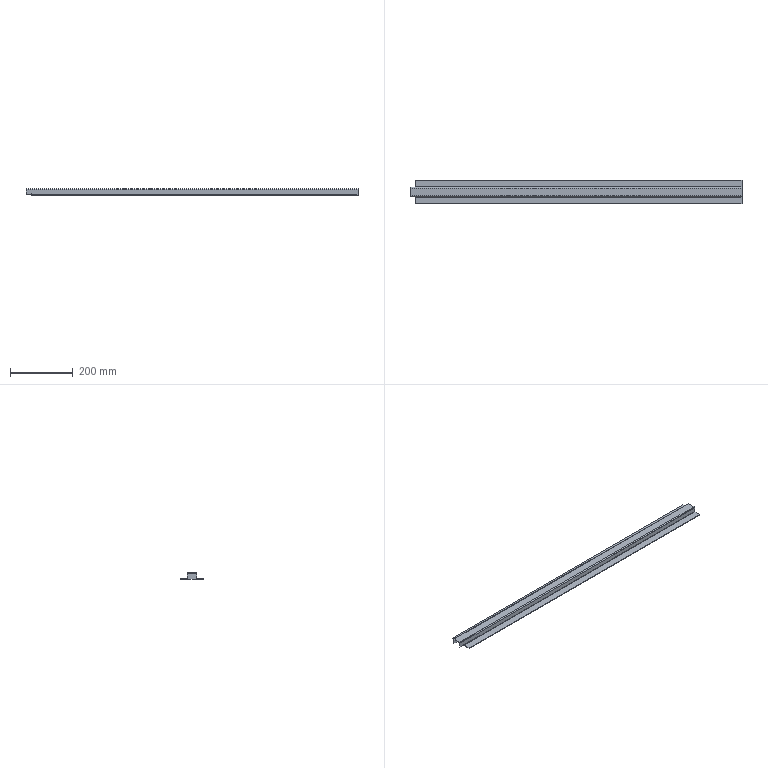Part | SolidWorks | features BaseBody 2 | 2 solids | 54 faces | box 1059 x 76 x 20 mm | volume 229133 mm3 | plane 44 | cylinder 10 | commonest cylinder face diameters 2 x6 6 x4
STEP:
#1=CARTESIAN_POINT('',(-529.5,-15.,-18.));
#2=VERTEX_POINT('',#1);
#3=CARTESIAN_POINT('',(-529.5,-13.,-18.));
#4=VERTEX_POINT('',#3);
#5=CARTESIAN_POINT('',(-529.5,-38.,-18.));
#6=DIRECTION('',(0.,1.,0.));
#7=VECTOR('',#6,1000.);
#8=LINE('',#5,#7);
#9=EDGE_CURVE('',#2,#4,#8,.T.);
#10=ORIENTED_EDGE('',*,*,#9,.T.);
#11=CARTESIAN_POINT('',(-512.5,-13.,-18.));
#12=VERTEX_POINT('',#11);
#13=CARTESIAN_POINT('',(0.,-13.,-18.));
#14=DIRECTION('',(1.,0.,0.));
#15=VECTOR('',#14,1000.);
#16=LINE('',#13,#15);
#17=EDGE_CURVE('',#4,#12,#16,.T.);
#18=ORIENTED_EDGE('',*,*,#17,.T.);
#19=CARTESIAN_POINT('',(-512.5,-15.,-18.));
#20=VERTEX_POINT('',#19);
#21=CARTESIAN_POINT('',(-512.5,-38.,-18.));
#22=DIRECTION('',(0.,1.,0.));
#23=VECTOR('',#22,1000.);
#24=LINE('',#21,#23);
#25=EDGE_CURVE('',#20,#12,#24,.T.);
#26=ORIENTED_EDGE('',*,*,#25,.F.);
#27=CARTESIAN_POINT('',(0.,-15.,-18.));
#28=DIRECTION('',(1.,0.,0.));
#29=VECTOR('',#28,1000.);
#30=LINE('',#27,#29);
#31=EDGE_CURVE('',#2,#20,#30,.T.);
#32=ORIENTED_EDGE('',*,*,#31,.F.);
#33=EDGE_LOOP('',(#10,#18,#26,#32));
#34=FACE_OUTER_BOUND('',#33,.T.);
#35=CARTESIAN_POINT('',(-529.5,-38.,-18.));
#36=DIRECTION('',(0.,0.,1.));
#37=DIRECTION('',(0.,-1.,0.));
#38=AXIS2_PLACEMENT_3D('',#35,#36,#37);
#39=PLANE('',#38);
#40=ADVANCED_FACE('',(#34),#39,.F.);
#41=CARTESIAN_POINT('',(-529.5,13.,-18.));
#42=VERTEX_POINT('',#41);
#43=CARTESIAN_POINT('',(-529.5,15.,-18.));
#44=VERTEX_POINT('',#43);
#45=CARTESIAN_POINT('',(-529.5,-38.,-18.));
#46=DIRECTION('',(0.,1.,0.));
#47=VECTOR('',#46,1000.);
#48=LINE('',#45,#47);
#49=EDGE_CURVE('',#42,#44,#48,.T.);
#50=ORIENTED_EDGE('',*,*,#49,.T.);
#51=CARTESIAN_POINT('',(-512.5,15.,-18.));
#52=VERTEX_POINT('',#51);
#53=CARTESIAN_POINT('',(-529.5,15.,-18.));
#54=DIRECTION('',(1.,0.,0.));
#55=VECTOR('',#54,1000.);
#56=LINE('',#53,#55);
#57=EDGE_CURVE('',#44,#52,#56,.T.);
#58=ORIENTED_EDGE('',*,*,#57,.T.);
#59=CARTESIAN_POINT('',(-512.5,13.,-18.));
#60=VERTEX_POINT('',#59);
#61=CARTESIAN_POINT('',(-512.5,15.,-18.));
#62=DIRECTION('',(0.,-1.,0.));
#63=VECTOR('',#62,1000.);
#64=LINE('',#61,#63);
#65=EDGE_CURVE('',#52,#60,#64,.T.);
#66=ORIENTED_EDGE('',*,*,#65,.T.);
#67=CARTESIAN_POINT('',(0.,13.,-18.));
#68=DIRECTION('',(1.,0.,0.));
#69=VECTOR('',#68,1000.);
#70=LINE('',#67,#69);
#71=EDGE_CURVE('',#42,#60,#70,.T.);
#72=ORIENTED_EDGE('',*,*,#71,.F.);
#73=EDGE_LOOP('',(#50,#58,#66,#72));
#74=FACE_OUTER_BOUND('',#73,.T.);
#75=CARTESIAN_POINT('',(-529.5,-38.,-18.));
#76=DIRECTION('',(0.,0.,1.));
#77=DIRECTION('',(0.,-1.,0.));
#78=AXIS2_PLACEMENT_3D('',#75,#76,#77);
#79=PLANE('',#78);
#80=ADVANCED_FACE('',(#74),#79,.F.);
#81=CARTESIAN_POINT('',(-511.5,38.,-18.));
#82=VERTEX_POINT('',#81);
#83=CARTESIAN_POINT('',(529.5,38.,-18.));
#84=VERTEX_POINT('',#83);
#85=CARTESIAN_POINT('',(529.5,38.,-18.));
#86=DIRECTION('',(1.,0.,0.));
#87=VECTOR('',#86,1000.);
#88=LINE('',#85,#87);
#89=EDGE_CURVE('',#82,#84,#88,.T.);
#90=ORIENTED_EDGE('',*,*,#89,.T.);
#91=CARTESIAN_POINT('',(529.5,38.,-20.));
#92=VERTEX_POINT('',#91);
#93=CARTESIAN_POINT('',(529.5,38.,-20.));
#94=DIRECTION('',(0.,0.,1.));
#95=VECTOR('',#94,1000.);
#96=LINE('',#93,#95);
#97=EDGE_CURVE('',#92,#84,#96,.T.);
#98=ORIENTED_EDGE('',*,*,#97,.F.);
#99=CARTESIAN_POINT('',(-511.5,38.,-20.));
#100=VERTEX_POINT('',#99);
#101=CARTESIAN_POINT('',(0.,38.,-20.));
#102=DIRECTION('',(1.,0.,0.));
#103=VECTOR('',#102,1000.);
#104=LINE('',#101,#103);
#105=EDGE_CURVE('',#100,#92,#104,.T.);
#106=ORIENTED_EDGE('',*,*,#105,.F.);
#107=CARTESIAN_POINT('',(-511.5,38.,-20.));
#108=DIRECTION('',(0.,0.,1.));
#109=VECTOR('',#108,1000.);
#110=LINE('',#107,#109);
#111=EDGE_CURVE('',#100,#82,#110,.T.);
#112=ORIENTED_EDGE('',*,*,#111,.T.);
#113=EDGE_LOOP('',(#90,#98,#106,#112));
#114=FACE_OUTER_BOUND('',#113,.T.);
#115=CARTESIAN_POINT('',(529.5,38.,-20.));
#116=DIRECTION('',(0.,-1.,0.));
#117=DIRECTION('',(-1.,0.,0.));
#118=AXIS2_PLACEMENT_3D('',#115,#116,#117);
#119=PLANE('',#118);
#120=ADVANCED_FACE('',(#114),#119,.F.);
#121=CARTESIAN_POINT('',(-511.5,16.,-18.));
#122=VERTEX_POINT('',#121);
#123=CARTESIAN_POINT('',(-511.5,15.,-18.));
#124=DIRECTION('',(0.,1.,0.));
#125=VECTOR('',#124,1000.);
#126=LINE('',#123,#125);
#127=EDGE_CURVE('',#122,#82,#126,.T.);
#128=ORIENTED_EDGE('',*,*,#127,.F.);
#129=CARTESIAN_POINT('',(529.5,16.,-18.));
#130=VERTEX_POINT('',#129);
#131=CARTESIAN_POINT('',(529.5,16.,-18.));
#132=DIRECTION('',(-1.,0.,0.));
#133=VECTOR('',#132,1000.);
#134=LINE('',#131,#133);
#135=EDGE_CURVE('',#130,#122,#134,.T.);
#136=ORIENTED_EDGE('',*,*,#135,.F.);
#137=CARTESIAN_POINT('',(529.5,15.,-18.));
#138=DIRECTION('',(0.,-1.,0.));
#139=VECTOR('',#138,1000.);
#140=LINE('',#137,#139);
#141=EDGE_CURVE('',#84,#130,#140,.T.);
#142=ORIENTED_EDGE('',*,*,#141,.F.);
#143=ORIENTED_EDGE('',*,*,#89,.F.);
#144=EDGE_LOOP('',(#128,#136,#142,#143));
#145=FACE_OUTER_BOUND('',#144,.T.);
#146=CARTESIAN_POINT('',(0.,0.,-18.));
#147=DIRECTION('',(0.,0.,1.));
#148=DIRECTION('',(1.,0.,0.));
#149=AXIS2_PLACEMENT_3D('',#146,#147,#148);
#150=PLANE('',#149);
#151=ADVANCED_FACE('',(#145),#150,.T.);
#152=CARTESIAN_POINT('',(-511.5,16.,-20.));
#153=VERTEX_POINT('',#152);
#154=CARTESIAN_POINT('',(529.5,16.,-20.));
#155=VERTEX_POINT('',#154);
#156=CARTESIAN_POINT('',(529.5,16.,-20.));
#157=DIRECTION('',(1.,0.,0.));
#158=VECTOR('',#157,1000.);
#159=LINE('',#156,#158);
#160=EDGE_CURVE('',#153,#155,#159,.T.);
#161=ORIENTED_EDGE('',*,*,#160,.F.);
#162=CARTESIAN_POINT('',(-511.5,0.,-20.));
#163=DIRECTION('',(0.,1.,0.));
#164=VECTOR('',#163,1000.);
#165=LINE('',#162,#164);
#166=EDGE_CURVE('',#153,#100,#165,.T.);
#167=ORIENTED_EDGE('',*,*,#166,.T.);
#168=ORIENTED_EDGE('',*,*,#105,.T.);
#169=CARTESIAN_POINT('',(529.5,0.,-20.));
#170=DIRECTION('',(0.,-1.,0.));
#171=VECTOR('',#170,1000.);
#172=LINE('',#169,#171);
#173=EDGE_CURVE('',#92,#155,#172,.T.);
#174=ORIENTED_EDGE('',*,*,#173,.T.);
#175=EDGE_LOOP('',(#161,#167,#168,#174));
#176=FACE_OUTER_BOUND('',#175,.T.);
#177=CARTESIAN_POINT('',(0.,0.,-20.));
#178=DIRECTION('',(0.,0.,1.));
#179=DIRECTION('',(1.,0.,0.));
#180=AXIS2_PLACEMENT_3D('',#177,#178,#179);
#181=PLANE('',#180);
#182=ADVANCED_FACE('',(#176),#181,.F.);
#183=CARTESIAN_POINT('',(-511.5,16.,-18.));
#184=DIRECTION('',(0.,0.,-1.));
#185=VECTOR('',#184,1000.);
#186=LINE('',#183,#185);
#187=EDGE_CURVE('',#122,#153,#186,.T.);
#188=ORIENTED_EDGE('',*,*,#187,.F.);
#189=ORIENTED_EDGE('',*,*,#127,.T.);
#190=ORIENTED_EDGE('',*,*,#111,.F.);
#191=ORIENTED_EDGE('',*,*,#166,.F.);
#192=EDGE_LOOP('',(#188,#189,#190,#191));
#193=FACE_OUTER_BOUND('',#192,.T.);
#194=CARTESIAN_POINT('',(-511.5,15.,-20.));
#195=DIRECTION('',(1.,0.,0.));
#196=DIRECTION('',(0.,1.,0.));
#197=AXIS2_PLACEMENT_3D('',#194,#195,#196);
#198=PLANE('',#197);
#199=ADVANCED_FACE('',(#193),#198,.F.);
#200=CARTESIAN_POINT('',(529.5,16.,-20.));
#201=DIRECTION('',(0.,0.,-1.));
#202=VECTOR('',#201,1000.);
#203=LINE('',#200,#202);
#204=EDGE_CURVE('',#130,#155,#203,.T.);
#205=ORIENTED_EDGE('',*,*,#204,.T.);
#206=ORIENTED_EDGE('',*,*,#173,.F.);
#207=ORIENTED_EDGE('',*,*,#97,.T.);
#208=ORIENTED_EDGE('',*,*,#141,.T.);
#209=EDGE_LOOP('',(#205,#206,#207,#208));
#210=FACE_OUTER_BOUND('',#209,.T.);
#211=CARTESIAN_POINT('',(529.5,15.,-20.));
#212=DIRECTION('',(-1.,0.,0.));
#213=DIRECTION('',(0.,0.,1.));
#214=AXIS2_PLACEMENT_3D('',#211,#212,#213);
#215=PLANE('',#214);
#216=ADVANCED_FACE('',(#210),#215,.F.);
#217=CARTESIAN_POINT('',(-511.5,15.,-17.));
#218=VERTEX_POINT('',#217);
#219=CARTESIAN_POINT('',(529.5,15.,-17.));
#220=VERTEX_POINT('',#219);
#221=CARTESIAN_POINT('',(-511.5,15.,-17.));
#222=DIRECTION('',(1.,0.,0.));
#223=VECTOR('',#222,1000.);
#224=LINE('',#221,#223);
#225=EDGE_CURVE('',#218,#220,#224,.T.);
#226=ORIENTED_EDGE('',*,*,#225,.T.);
#227=CARTESIAN_POINT('',(529.5,16.,-17.));
#228=DIRECTION('',(1.,0.,0.));
#229=DIRECTION('',(0.,0.,1.));
#230=AXIS2_PLACEMENT_3D('',#227,#228,#229);
#231=CIRCLE('',#230,1.);
#232=EDGE_CURVE('',#220,#130,#231,.T.);
#233=ORIENTED_EDGE('',*,*,#232,.T.);
#234=ORIENTED_EDGE('',*,*,#135,.T.);
#235=CARTESIAN_POINT('',(-511.5,16.,-17.));
#236=DIRECTION('',(-1.,0.,0.));
#237=DIRECTION('',(0.,0.,1.));
#238=AXIS2_PLACEMENT_3D('',#235,#236,#237);
#239=CIRCLE('',#238,1.);
#240=EDGE_CURVE('',#122,#218,#239,.T.);
#241=ORIENTED_EDGE('',*,*,#240,.T.);
#242=EDGE_LOOP('',(#226,#233,#234,#241));
#243=FACE_OUTER_BOUND('',#242,.T.);
#244=CARTESIAN_POINT('',(-511.5,16.,-17.));
#245=DIRECTION('',(-1.,0.,0.));
#246=DIRECTION('',(0.,0.,-1.));
#247=AXIS2_PLACEMENT_3D('',#244,#245,#246);
#248=CYLINDRICAL_SURFACE('',#247,1.);
#249=ADVANCED_FACE('',(#243),#248,.F.);
#250=CARTESIAN_POINT('',(-511.5,13.,-17.));
#251=VERTEX_POINT('',#250);
#252=CARTESIAN_POINT('',(529.5,13.,-17.));
#253=VERTEX_POINT('',#252);
#254=CARTESIAN_POINT('',(-511.5,13.,-17.));
#255=DIRECTION('',(1.,0.,0.));
#256=VECTOR('',#255,1000.);
#257=LINE('',#254,#256);
#258=EDGE_CURVE('',#251,#253,#257,.T.);
#259=ORIENTED_EDGE('',*,*,#258,.F.);
#260=CARTESIAN_POINT('',(-511.5,16.,-17.));
#261=DIRECTION('',(-1.,0.,0.));
#262=DIRECTION('',(0.,0.,1.));
#263=AXIS2_PLACEMENT_3D('',#260,#261,#262);
#264=CIRCLE('',#263,3.);
#265=EDGE_CURVE('',#153,#251,#264,.T.);
#266=ORIENTED_EDGE('',*,*,#265,.F.);
#267=ORIENTED_EDGE('',*,*,#160,.T.);
#268=CARTESIAN_POINT('',(529.5,16.,-17.));
#269=DIRECTION('',(1.,0.,0.));
#270=DIRECTION('',(0.,0.,1.));
#271=AXIS2_PLACEMENT_3D('',#268,#269,#270);
#272=CIRCLE('',#271,3.);
#273=EDGE_CURVE('',#253,#155,#272,.T.);
#274=ORIENTED_EDGE('',*,*,#273,.F.);
#275=EDGE_LOOP('',(#259,#266,#267,#274));
#276=FACE_OUTER_BOUND('',#275,.T.);
#277=CARTESIAN_POINT('',(-511.5,16.,-17.));
#278=DIRECTION('',(-1.,0.,0.));
#279=DIRECTION('',(0.,0.,-1.));
#280=AXIS2_PLACEMENT_3D('',#277,#278,#279);
#281=CYLINDRICAL_SURFACE('',#280,3.);
#282=ADVANCED_FACE('',(#276),#281,.T.);
#283=ORIENTED_EDGE('',*,*,#240,.F.);
#284=ORIENTED_EDGE('',*,*,#187,.T.);
#285=ORIENTED_EDGE('',*,*,#265,.T.);
#286=CARTESIAN_POINT('',(-511.5,15.,-17.));
#287=DIRECTION('',(0.,-1.,0.));
#288=VECTOR('',#287,1000.);
#289=LINE('',#286,#288);
#290=EDGE_CURVE('',#218,#251,#289,.T.);
#291=ORIENTED_EDGE('',*,*,#290,.F.);
#292=EDGE_LOOP('',(#283,#284,#285,#291));
#293=FACE_OUTER_BOUND('',#292,.T.);
#294=CARTESIAN_POINT('',(-511.5,16.,-17.));
#295=DIRECTION('',(1.,0.,0.));
#296=DIRECTION('',(0.,1.,0.));
#297=AXIS2_PLACEMENT_3D('',#294,#295,#296);
#298=PLANE('',#297);
#299=ADVANCED_FACE('',(#293),#298,.F.);
#300=ORIENTED_EDGE('',*,*,#204,.F.);
#301=ORIENTED_EDGE('',*,*,#232,.F.);
#302=CARTESIAN_POINT('',(529.5,15.,-17.));
#303=DIRECTION('',(0.,-1.,0.));
#304=VECTOR('',#303,1000.);
#305=LINE('',#302,#304);
#306=EDGE_CURVE('',#220,#253,#305,.T.);
#307=ORIENTED_EDGE('',*,*,#306,.T.);
#308=ORIENTED_EDGE('',*,*,#273,.T.);
#309=EDGE_LOOP('',(#300,#301,#307,#308));
#310=FACE_OUTER_BOUND('',#309,.T.);
#311=CARTESIAN_POINT('',(529.5,16.,-17.));
#312=DIRECTION('',(1.,0.,0.));
#313=DIRECTION('',(0.,1.,0.));
#314=AXIS2_PLACEMENT_3D('',#311,#312,#313);
#315=PLANE('',#314);
#316=ADVANCED_FACE('',(#310),#315,.T.);
#317=ORIENTED_EDGE('',*,*,#65,.F.);
#318=CARTESIAN_POINT('',(-512.5,15.,-16.));
#319=VERTEX_POINT('',#318);
#320=CARTESIAN_POINT('',(-512.5,15.,-20.));
#321=DIRECTION('',(0.,0.,1.));
#322=VECTOR('',#321,1000.);
#323=LINE('',#320,#322);
#324=EDGE_CURVE('',#52,#319,#323,.T.);
#325=ORIENTED_EDGE('',*,*,#324,.T.);
#326=CARTESIAN_POINT('',(-512.5,13.,-16.));
#327=VERTEX_POINT('',#326);
#328=CARTESIAN_POINT('',(-512.5,15.,-16.));
#329=DIRECTION('',(0.,-1.,0.));
#330=VECTOR('',#329,1000.);
#331=LINE('',#328,#330);
#332=EDGE_CURVE('',#319,#327,#331,.T.);
#333=ORIENTED_EDGE('',*,*,#332,.T.);
#334=CARTESIAN_POINT('',(-512.5,13.,0.));
#335=DIRECTION('',(0.,0.,-1.));
#336=VECTOR('',#335,1000.);
#337=LINE('',#334,#336);
#338=EDGE_CURVE('',#327,#60,#337,.T.);
#339=ORIENTED_EDGE('',*,*,#338,.T.);
#340=EDGE_LOOP('',(#317,#325,#333,#339));
#341=FACE_OUTER_BOUND('',#340,.T.);
#342=CARTESIAN_POINT('',(-512.5,15.,-20.));
#343=DIRECTION('',(1.,0.,0.));
#344=DIRECTION('',(0.,0.,1.));
#345=AXIS2_PLACEMENT_3D('',#342,#343,#344);
#346=PLANE('',#345);
#347=ADVANCED_FACE('',(#341),#346,.T.);
#348=ORIENTED_EDGE('',*,*,#290,.T.);
#349=CARTESIAN_POINT('',(-511.5,13.,-16.));
#350=VERTEX_POINT('',#349);
#351=CARTESIAN_POINT('',(-511.5,13.,0.));
#352=DIRECTION('',(0.,0.,1.));
#353=VECTOR('',#352,1000.);
#354=LINE('',#351,#353);
#355=EDGE_CURVE('',#251,#350,#354,.T.);
#356=ORIENTED_EDGE('',*,*,#355,.T.);
#357=CARTESIAN_POINT('',(-511.5,15.,-16.));
#358=VERTEX_POINT('',#357);
#359=CARTESIAN_POINT('',(-511.5,15.,-16.));
#360=DIRECTION('',(0.,-1.,0.));
#361=VECTOR('',#360,1000.);
#362=LINE('',#359,#361);
#363=EDGE_CURVE('',#358,#350,#362,.T.);
#364=ORIENTED_EDGE('',*,*,#363,.F.);
#365=CARTESIAN_POINT('',(-511.5,15.,-16.));
#366=DIRECTION('',(0.,0.,-1.));
#367=VECTOR('',#366,1000.);
#368=LINE('',#365,#367);
#369=EDGE_CURVE('',#358,#218,#368,.T.);
#370=ORIENTED_EDGE('',*,*,#369,.T.);
#371=EDGE_LOOP('',(#348,#356,#364,#370));
#372=FACE_OUTER_BOUND('',#371,.T.);
#373=CARTESIAN_POINT('',(-511.5,15.,-16.));
#374=DIRECTION('',(-1.,0.,0.));
#375=DIRECTION('',(0.,0.,1.));
#376=AXIS2_PLACEMENT_3D('',#373,#374,#375);
#377=PLANE('',#376);
#378=ADVANCED_FACE('',(#372),#377,.T.);
#379=ORIENTED_EDGE('',*,*,#363,.T.);
#380=CARTESIAN_POINT('',(0.,13.,-16.));
#381=DIRECTION('',(-1.,0.,0.));
#382=VECTOR('',#381,1000.);
#383=LINE('',#380,#382);
#384=EDGE_CURVE('',#350,#327,#383,.T.);
#385=ORIENTED_EDGE('',*,*,#384,.T.);
#386=ORIENTED_EDGE('',*,*,#332,.F.);
#387=CARTESIAN_POINT('',(-512.5,15.,-16.));
#388=DIRECTION('',(1.,0.,0.));
#389=VECTOR('',#388,1000.);
#390=LINE('',#387,#389);
#391=EDGE_CURVE('',#319,#358,#390,.T.);
#392=ORIENTED_EDGE('',*,*,#391,.T.);
#393=EDGE_LOOP('',(#379,#385,#386,#392));
#394=FACE_OUTER_BOUND('',#393,.T.);
#395=CARTESIAN_POINT('',(-512.5,15.,-16.));
#396=DIRECTION('',(0.,0.,-1.));
#397=DIRECTION('',(-1.,0.,0.));
#398=AXIS2_PLACEMENT_3D('',#395,#396,#397);
#399=PLANE('',#398);
#400=ADVANCED_FACE('',(#394),#399,.T.);
#401=CARTESIAN_POINT('',(-511.5,-38.,-18.));
#402=VERTEX_POINT('',#401);
#403=CARTESIAN_POINT('',(529.5,-38.,-18.));
#404=VERTEX_POINT('',#403);
#405=CARTESIAN_POINT('',(0.,-38.,-18.));
#406=DIRECTION('',(1.,0.,0.));
#407=VECTOR('',#406,1000.);
#408=LINE('',#405,#407);
#409=EDGE_CURVE('',#402,#404,#408,.T.);
#410=ORIENTED_EDGE('',*,*,#409,.F.);
#411=CARTESIAN_POINT('',(-511.5,-38.,-20.));
#412=VERTEX_POINT('',#411);
#413=CARTESIAN_POINT('',(-511.5,-38.,-20.));
#414=DIRECTION('',(0.,0.,1.));
#415=VECTOR('',#414,1000.);
#416=LINE('',#413,#415);
#417=EDGE_CURVE('',#412,#402,#416,.T.);
#418=ORIENTED_EDGE('',*,*,#417,.F.);
#419=CARTESIAN_POINT('',(529.5,-38.,-20.));
#420=VERTEX_POINT('',#419);
#421=CARTESIAN_POINT('',(-511.5,-38.,-20.));
#422=DIRECTION('',(1.,0.,0.));
#423=VECTOR('',#422,1000.);
#424=LINE('',#421,#423);
#425=EDGE_CURVE('',#412,#420,#424,.T.);
#426=ORIENTED_EDGE('',*,*,#425,.T.);
#427=CARTESIAN_POINT('',(529.5,-38.,-20.));
#428=DIRECTION('',(0.,0.,1.));
#429=VECTOR('',#428,1000.);
#430=LINE('',#427,#429);
#431=EDGE_CURVE('',#420,#404,#430,.T.);
#432=ORIENTED_EDGE('',*,*,#431,.T.);
#433=EDGE_LOOP('',(#410,#418,#426,#432));
#434=FACE_OUTER_BOUND('',#433,.T.);
#435=CARTESIAN_POINT('',(-511.5,-38.,-20.));
#436=DIRECTION('',(0.,-1.,0.));
#437=DIRECTION('',(0.,0.,-1.));
#438=AXIS2_PLACEMENT_3D('',#435,#436,#437);
#439=PLANE('',#438);
#440=ADVANCED_FACE('',(#434),#439,.T.);
#441=CARTESIAN_POINT('',(-511.5,-16.,-18.));
#442=VERTEX_POINT('',#441);
#443=CARTESIAN_POINT('',(529.5,-16.,-18.));
#444=VERTEX_POINT('',#443);
#445=CARTESIAN_POINT('',(-511.5,-16.,-18.));
#446=DIRECTION('',(1.,0.,0.));
#447=VECTOR('',#446,1000.);
#448=LINE('',#445,#447);
#449=EDGE_CURVE('',#442,#444,#448,.T.);
#450=ORIENTED_EDGE('',*,*,#449,.F.);
#451=CARTESIAN_POINT('',(-511.5,0.,-18.));
#452=DIRECTION('',(0.,-1.,0.));
#453=VECTOR('',#452,1000.);
#454=LINE('',#451,#453);
#455=EDGE_CURVE('',#442,#402,#454,.T.);
#456=ORIENTED_EDGE('',*,*,#455,.T.);
#457=ORIENTED_EDGE('',*,*,#409,.T.);
#458=CARTESIAN_POINT('',(529.5,0.,-18.));
#459=DIRECTION('',(0.,1.,0.));
#460=VECTOR('',#459,1000.);
#461=LINE('',#458,#460);
#462=EDGE_CURVE('',#404,#444,#461,.T.);
#463=ORIENTED_EDGE('',*,*,#462,.T.);
#464=EDGE_LOOP('',(#450,#456,#457,#463));
#465=FACE_OUTER_BOUND('',#464,.T.);
#466=CARTESIAN_POINT('',(0.,0.,-18.));
#467=DIRECTION('',(0.,0.,-1.));
#468=DIRECTION('',(-1.,0.,0.));
#469=AXIS2_PLACEMENT_3D('',#466,#467,#468);
#470=PLANE('',#469);
#471=ADVANCED_FACE('',(#465),#470,.F.);
#472=CARTESIAN_POINT('',(-511.5,-16.,-20.));
#473=VERTEX_POINT('',#472);
#474=CARTESIAN_POINT('',(-511.5,-15.,-20.));
#475=DIRECTION('',(0.,-1.,0.));
#476=VECTOR('',#475,1000.);
#477=LINE('',#474,#476);
#478=EDGE_CURVE('',#473,#412,#477,.T.);
#479=ORIENTED_EDGE('',*,*,#478,.F.);
#480=CARTESIAN_POINT('',(529.5,-16.,-20.));
#481=VERTEX_POINT('',#480);
#482=CARTESIAN_POINT('',(0.,-16.,-20.));
#483=DIRECTION('',(1.,0.,0.));
#484=VECTOR('',#483,1000.);
#485=LINE('',#482,#484);
#486=EDGE_CURVE('',#473,#481,#485,.T.);
#487=ORIENTED_EDGE('',*,*,#486,.T.);
#488=CARTESIAN_POINT('',(529.5,-38.,-20.));
#489=DIRECTION('',(0.,1.,0.));
#490=VECTOR('',#489,1000.);
#491=LINE('',#488,#490);
#492=EDGE_CURVE('',#420,#481,#491,.T.);
#493=ORIENTED_EDGE('',*,*,#492,.F.);
#494=ORIENTED_EDGE('',*,*,#425,.F.);
#495=EDGE_LOOP('',(#479,#487,#493,#494));
#496=FACE_OUTER_BOUND('',#495,.T.);
#497=CARTESIAN_POINT('',(0.,0.,-20.));
#498=DIRECTION('',(0.,0.,-1.));
#499=DIRECTION('',(-1.,0.,0.));
#500=AXIS2_PLACEMENT_3D('',#497,#498,#499);
#501=PLANE('',#500);
#502=ADVANCED_FACE('',(#496),#501,.T.);
#503=ORIENTED_EDGE('',*,*,#455,.F.);
#504=CARTESIAN_POINT('',(-511.5,-16.,-20.));
#505=DIRECTION('',(0.,0.,-1.));
#506=VECTOR('',#505,1000.);
#507=LINE('',#504,#506);
#508=EDGE_CURVE('',#442,#473,#507,.T.);
#509=ORIENTED_EDGE('',*,*,#508,.T.);
#510=ORIENTED_EDGE('',*,*,#478,.T.);
#511=ORIENTED_EDGE('',*,*,#417,.T.);
#512=EDGE_LOOP('',(#503,#509,#510,#511));
#513=FACE_OUTER_BOUND('',#512,.T.);
#514=CARTESIAN_POINT('',(-511.5,-15.,-20.));
#515=DIRECTION('',(-1.,0.,0.));
#516=DIRECTION('',(0.,1.,0.));
#517=AXIS2_PLACEMENT_3D('',#514,#515,#516);
#518=PLANE('',#517);
#519=ADVANCED_FACE('',(#513),#518,.T.);
#520=ORIENTED_EDGE('',*,*,#492,.T.);
#521=CARTESIAN_POINT('',(529.5,-16.,-18.));
#522=DIRECTION('',(0.,0.,-1.));
#523=VECTOR('',#522,1000.);
#524=LINE('',#521,#523);
#525=EDGE_CURVE('',#444,#481,#524,.T.);
#526=ORIENTED_EDGE('',*,*,#525,.F.);
#527=ORIENTED_EDGE('',*,*,#462,.F.);
#528=ORIENTED_EDGE('',*,*,#431,.F.);
#529=EDGE_LOOP('',(#520,#526,#527,#528));
#530=FACE_OUTER_BOUND('',#529,.T.);
#531=CARTESIAN_POINT('',(529.5,-38.,-20.));
#532=DIRECTION('',(1.,0.,0.));
#533=DIRECTION('',(0.,0.,-1.));
#534=AXIS2_PLACEMENT_3D('',#531,#532,#533);
#535=PLANE('',#534);
#536=ADVANCED_FACE('',(#530),#535,.T.);
#537=CARTESIAN_POINT('',(529.5,-15.,-17.));
#538=VERTEX_POINT('',#537);
#539=CARTESIAN_POINT('',(-511.5,-15.,-17.));
#540=VERTEX_POINT('',#539);
#541=CARTESIAN_POINT('',(529.5,-15.,-17.));
#542=DIRECTION('',(-1.,0.,0.));
#543=VECTOR('',#542,1000.);
#544=LINE('',#541,#543);
#545=EDGE_CURVE('',#538,#540,#544,.T.);
#546=ORIENTED_EDGE('',*,*,#545,.T.);
#547=CARTESIAN_POINT('',(-511.5,-16.,-17.));
#548=DIRECTION('',(-1.,0.,0.));
#549=DIRECTION('',(0.,0.,-1.));
#550=AXIS2_PLACEMENT_3D('',#547,#548,#549);
#551=CIRCLE('',#550,1.);
#552=EDGE_CURVE('',#540,#442,#551,.T.);
#553=ORIENTED_EDGE('',*,*,#552,.T.);
#554=ORIENTED_EDGE('',*,*,#449,.T.);
#555=CARTESIAN_POINT('',(529.5,-16.,-17.));
#556=DIRECTION('',(1.,0.,0.));
#557=DIRECTION('',(0.,0.,-1.));
#558=AXIS2_PLACEMENT_3D('',#555,#556,#557);
#559=CIRCLE('',#558,1.);
#560=EDGE_CURVE('',#444,#538,#559,.T.);
#561=ORIENTED_EDGE('',*,*,#560,.T.);
#562=EDGE_LOOP('',(#546,#553,#554,#561));
#563=FACE_OUTER_BOUND('',#562,.T.);
#564=CARTESIAN_POINT('',(529.5,-16.,-17.));
#565=DIRECTION('',(1.,0.,0.));
#566=DIRECTION('',(0.,0.,-1.));
#567=AXIS2_PLACEMENT_3D('',#564,#565,#566);
#568=CYLINDRICAL_SURFACE('',#567,1.);
#569=ADVANCED_FACE('',(#563),#568,.F.);
#570=CARTESIAN_POINT('',(529.5,-13.,-17.));
#571=VERTEX_POINT('',#570);
#572=CARTESIAN_POINT('',(-511.5,-13.,-17.));
#573=VERTEX_POINT('',#572);
#574=CARTESIAN_POINT('',(529.5,-13.,-17.));
#575=DIRECTION('',(-1.,0.,0.));
#576=VECTOR('',#575,1000.);
#577=LINE('',#574,#576);
#578=EDGE_CURVE('',#571,#573,#577,.T.);
#579=ORIENTED_EDGE('',*,*,#578,.F.);
#580=CARTESIAN_POINT('',(529.5,-16.,-17.));
#581=DIRECTION('',(1.,0.,0.));
#582=DIRECTION('',(0.,0.,-1.));
#583=AXIS2_PLACEMENT_3D('',#580,#581,#582);
#584=CIRCLE('',#583,3.);
#585=EDGE_CURVE('',#481,#571,#584,.T.);
#586=ORIENTED_EDGE('',*,*,#585,.F.);
#587=ORIENTED_EDGE('',*,*,#486,.F.);
#588=CARTESIAN_POINT('',(-511.5,-16.,-17.));
#589=DIRECTION('',(-1.,0.,0.));
#590=DIRECTION('',(0.,0.,-1.));
#591=AXIS2_PLACEMENT_3D('',#588,#589,#590);
#592=CIRCLE('',#591,3.);
#593=EDGE_CURVE('',#573,#473,#592,.T.);
#594=ORIENTED_EDGE('',*,*,#593,.F.);
#595=EDGE_LOOP('',(#579,#586,#587,#594));
#596=FACE_OUTER_BOUND('',#595,.T.);
#597=CARTESIAN_POINT('',(529.5,-16.,-17.));
#598=DIRECTION('',(1.,0.,0.));
#599=DIRECTION('',(0.,0.,-1.));
#600=AXIS2_PLACEMENT_3D('',#597,#598,#599);
#601=CYLINDRICAL_SURFACE('',#600,3.);
#602=ADVANCED_FACE('',(#596),#601,.T.);
#603=ORIENTED_EDGE('',*,*,#560,.F.);
#604=ORIENTED_EDGE('',*,*,#525,.T.);
#605=ORIENTED_EDGE('',*,*,#585,.T.);
#606=CARTESIAN_POINT('',(529.5,-15.,-17.));
#607=DIRECTION('',(0.,1.,0.));
#608=VECTOR('',#607,1000.);
#609=LINE('',#606,#608);
#610=EDGE_CURVE('',#538,#571,#609,.T.);
#611=ORIENTED_EDGE('',*,*,#610,.F.);
#612=EDGE_LOOP('',(#603,#604,#605,#611));
#613=FACE_OUTER_BOUND('',#612,.T.);
#614=CARTESIAN_POINT('',(529.5,-16.,-17.));
#615=DIRECTION('',(-1.,0.,0.));
#616=DIRECTION('',(0.,0.,1.));
#617=AXIS2_PLACEMENT_3D('',#614,#615,#616);
#618=PLANE('',#617);
#619=ADVANCED_FACE('',(#613),#618,.F.);
#620=ORIENTED_EDGE('',*,*,#508,.F.);
#621=ORIENTED_EDGE('',*,*,#552,.F.);
#622=CARTESIAN_POINT('',(-511.5,-15.,-17.));
#623=DIRECTION('',(0.,1.,0.));
#624=VECTOR('',#623,1000.);
#625=LINE('',#622,#624);
#626=EDGE_CURVE('',#540,#573,#625,.T.);
#627=ORIENTED_EDGE('',*,*,#626,.T.);
#628=ORIENTED_EDGE('',*,*,#593,.T.);
#629=EDGE_LOOP('',(#620,#621,#627,#628));
#630=FACE_OUTER_BOUND('',#629,.T.);
#631=CARTESIAN_POINT('',(-511.5,-16.,-17.));
#632=DIRECTION('',(-1.,0.,0.));
#633=DIRECTION('',(0.,0.,1.));
#634=AXIS2_PLACEMENT_3D('',#631,#632,#633);
#635=PLANE('',#634);
#636=ADVANCED_FACE('',(#630),#635,.T.);
#637=ORIENTED_EDGE('',*,*,#25,.T.);
#638=CARTESIAN_POINT('',(-512.5,-13.,-16.));
#639=VERTEX_POINT('',#638);
#640=CARTESIAN_POINT('',(-512.5,-13.,0.));
#641=DIRECTION('',(0.,0.,-1.));
#642=VECTOR('',#641,1000.);
#643=LINE('',#640,#642);
#644=EDGE_CURVE('',#639,#12,#643,.T.);
#645=ORIENTED_EDGE('',*,*,#644,.F.);
#646=CARTESIAN_POINT('',(-512.5,-15.,-16.));
#647=VERTEX_POINT('',#646);
#648=CARTESIAN_POINT('',(-512.5,-15.,-16.));
#649=DIRECTION('',(0.,1.,0.));
#650=VECTOR('',#649,1000.);
#651=LINE('',#648,#650);
#652=EDGE_CURVE('',#647,#639,#651,.T.);
#653=ORIENTED_EDGE('',*,*,#652,.F.);
#654=CARTESIAN_POINT('',(-512.5,-15.,-16.));
#655=DIRECTION('',(0.,0.,-1.));
#656=VECTOR('',#655,1000.);
#657=LINE('',#654,#656);
#658=EDGE_CURVE('',#647,#20,#657,.T.);
#659=ORIENTED_EDGE('',*,*,#658,.T.);
#660=EDGE_LOOP('',(#637,#645,#653,#659));
#661=FACE_OUTER_BOUND('',#660,.T.);
#662=CARTESIAN_POINT('',(-512.5,-15.,-16.));
#663=DIRECTION('',(1.,0.,0.));
#664=DIRECTION('',(0.,0.,1.));
#665=AXIS2_PLACEMENT_3D('',#662,#663,#664);
#666=PLANE('',#665);
#667=ADVANCED_FACE('',(#661),#666,.T.);
#668=CARTESIAN_POINT('',(-511.5,-13.,-16.));
#669=VERTEX_POINT('',#668);
#670=CARTESIAN_POINT('',(0.,-13.,-16.));
#671=DIRECTION('',(-1.,0.,0.));
#672=VECTOR('',#671,1000.);
#673=LINE('',#670,#672);
#674=EDGE_CURVE('',#669,#639,#673,.T.);
#675=ORIENTED_EDGE('',*,*,#674,.F.);
#676=CARTESIAN_POINT('',(-511.5,-15.,-16.));
#677=VERTEX_POINT('',#676);
#678=CARTESIAN_POINT('',(-511.5,-15.,-16.));
#679=DIRECTION('',(0.,1.,0.));
#680=VECTOR('',#679,1000.);
#681=LINE('',#678,#680);
#682=EDGE_CURVE('',#677,#669,#681,.T.);
#683=ORIENTED_EDGE('',*,*,#682,.F.);
#684=CARTESIAN_POINT('',(-511.5,-15.,-16.));
#685=DIRECTION('',(-1.,0.,0.));
#686=VECTOR('',#685,1000.);
#687=LINE('',#684,#686);
#688=EDGE_CURVE('',#677,#647,#687,.T.);
#689=ORIENTED_EDGE('',*,*,#688,.T.);
#690=ORIENTED_EDGE('',*,*,#652,.T.);
#691=EDGE_LOOP('',(#675,#683,#689,#690));
#692=FACE_OUTER_BOUND('',#691,.T.);
#693=CARTESIAN_POINT('',(-511.5,-15.,-16.));
#694=DIRECTION('',(0.,0.,-1.));
#695=DIRECTION('',(0.,-1.,0.));
#696=AXIS2_PLACEMENT_3D('',#693,#694,#695);
#697=PLANE('',#696);
#698=ADVANCED_FACE('',(#692),#697,.T.);
#699=CARTESIAN_POINT('',(-511.5,-13.,0.));
#700=DIRECTION('',(0.,0.,1.));
#701=VECTOR('',#700,1000.);
#702=LINE('',#699,#701);
#703=EDGE_CURVE('',#573,#669,#702,.T.);
#704=ORIENTED_EDGE('',*,*,#703,.F.);
#705=ORIENTED_EDGE('',*,*,#626,.F.);
#706=CARTESIAN_POINT('',(-511.5,-15.,-17.));
#707=DIRECTION('',(0.,0.,1.));
#708=VECTOR('',#707,1000.);
#709=LINE('',#706,#708);
#710=EDGE_CURVE('',#540,#677,#709,.T.);
#711=ORIENTED_EDGE('',*,*,#710,.T.);
#712=ORIENTED_EDGE('',*,*,#682,.T.);
#713=EDGE_LOOP('',(#704,#705,#711,#712));
#714=FACE_OUTER_BOUND('',#713,.T.);
#715=CARTESIAN_POINT('',(-511.5,-15.,-17.));
#716=DIRECTION('',(-1.,0.,0.));
#717=DIRECTION('',(0.,1.,0.));
#718=AXIS2_PLACEMENT_3D('',#715,#716,#717);
#719=PLANE('',#718);
#720=ADVANCED_FACE('',(#714),#719,.T.);
#721=ORIENTED_EDGE('',*,*,#9,.F.);
#722=CARTESIAN_POINT('',(-529.5,-15.,-3.));
#723=VERTEX_POINT('',#722);
#724=CARTESIAN_POINT('',(-529.5,-15.,-20.));
#725=DIRECTION('',(0.,0.,1.));
#726=VECTOR('',#725,1000.);
#727=LINE('',#724,#726);
#728=EDGE_CURVE('',#2,#723,#727,.T.);
#729=ORIENTED_EDGE('',*,*,#728,.T.);
#730=CARTESIAN_POINT('',(-529.5,-13.,-3.));
#731=VERTEX_POINT('',#730);
#732=CARTESIAN_POINT('',(-529.5,-13.,-3.));
#733=DIRECTION('',(0.,-1.,0.));
#734=VECTOR('',#733,1000.);
#735=LINE('',#732,#734);
#736=EDGE_CURVE('',#731,#723,#735,.T.);
#737=ORIENTED_EDGE('',*,*,#736,.F.);
#738=CARTESIAN_POINT('',(-529.5,-13.,0.));
#739=DIRECTION('',(0.,0.,1.));
#740=VECTOR('',#739,1000.);
#741=LINE('',#738,#740);
#742=EDGE_CURVE('',#4,#731,#741,.T.);
#743=ORIENTED_EDGE('',*,*,#742,.F.);
#744=EDGE_LOOP('',(#721,#729,#737,#743));
#745=FACE_OUTER_BOUND('',#744,.T.);
#746=CARTESIAN_POINT('',(-529.5,-15.,-20.));
#747=DIRECTION('',(-1.,0.,0.));
#748=DIRECTION('',(0.,0.,1.));
#749=AXIS2_PLACEMENT_3D('',#746,#747,#748);
#750=PLANE('',#749);
#751=ADVANCED_FACE('',(#745),#750,.T.);
#752=CARTESIAN_POINT('',(-529.5,-12.,-2.));
#753=VERTEX_POINT('',#752);
#754=CARTESIAN_POINT('',(529.5,-12.,-2.));
#755=VERTEX_POINT('',#754);
#756=CARTESIAN_POINT('',(-529.5,-12.,-2.));
#757=DIRECTION('',(1.,0.,0.));
#758=VECTOR('',#757,1000.);
#759=LINE('',#756,#758);
#760=EDGE_CURVE('',#753,#755,#759,.T.);
#761=ORIENTED_EDGE('',*,*,#760,.T.);
#762=CARTESIAN_POINT('',(529.5,-13.,-3.));
#763=VERTEX_POINT('',#762);
#764=CARTESIAN_POINT('',(529.5,-12.,-3.));
#765=DIRECTION('',(1.,0.,0.));
#766=DIRECTION('',(0.,0.,1.));
#767=AXIS2_PLACEMENT_3D('',#764,#765,#766);
#768=CIRCLE('',#767,1.);
#769=EDGE_CURVE('',#755,#763,#768,.T.);
#770=ORIENTED_EDGE('',*,*,#769,.T.);
#771=CARTESIAN_POINT('',(529.5,-13.,-3.));
#772=DIRECTION('',(-1.,0.,0.));
#773=VECTOR('',#772,1000.);
#774=LINE('',#771,#773);
#775=EDGE_CURVE('',#763,#731,#774,.T.);
#776=ORIENTED_EDGE('',*,*,#775,.T.);
#777=CARTESIAN_POINT('',(-529.5,-12.,-3.));
#778=DIRECTION('',(-1.,0.,0.));
#779=DIRECTION('',(0.,0.,1.));
#780=AXIS2_PLACEMENT_3D('',#777,#778,#779);
#781=CIRCLE('',#780,1.);
#782=EDGE_CURVE('',#731,#753,#781,.T.);
#783=ORIENTED_EDGE('',*,*,#782,.T.);
#784=EDGE_LOOP('',(#761,#770,#776,#783));
#785=FACE_OUTER_BOUND('',#784,.T.);
#786=CARTESIAN_POINT('',(-529.5,-12.,-3.));
#787=DIRECTION('',(-1.,0.,0.));
#788=DIRECTION('',(0.,-1.,0.));
#789=AXIS2_PLACEMENT_3D('',#786,#787,#788);
#790=CYLINDRICAL_SURFACE('',#789,1.);
#791=ADVANCED_FACE('',(#785),#790,.F.);
#792=CARTESIAN_POINT('',(-529.5,-12.,0.));
#793=VERTEX_POINT('',#792);
#794=CARTESIAN_POINT('',(529.5,-12.,0.));
#795=VERTEX_POINT('',#794);
#796=CARTESIAN_POINT('',(-529.5,-12.,0.));
#797=DIRECTION('',(1.,0.,0.));
#798=VECTOR('',#797,1000.);
#799=LINE('',#796,#798);
#800=EDGE_CURVE('',#793,#795,#799,.T.);
#801=ORIENTED_EDGE('',*,*,#800,.F.);
#802=CARTESIAN_POINT('',(-529.5,-12.,-3.));
#803=DIRECTION('',(-1.,0.,0.));
#804=DIRECTION('',(0.,0.,1.));
#805=AXIS2_PLACEMENT_3D('',#802,#803,#804);
#806=CIRCLE('',#805,3.);
#807=EDGE_CURVE('',#723,#793,#806,.T.);
#808=ORIENTED_EDGE('',*,*,#807,.F.);
#809=CARTESIAN_POINT('',(529.5,-15.,-3.));
#810=VERTEX_POINT('',#809);
#811=CARTESIAN_POINT('',(529.5,-15.,-3.));
#812=DIRECTION('',(1.,0.,0.));
#813=VECTOR('',#812,1000.);
#814=LINE('',#811,#813);
#815=EDGE_CURVE('',#723,#810,#814,.T.);
#816=ORIENTED_EDGE('',*,*,#815,.T.);
#817=CARTESIAN_POINT('',(529.5,-12.,-3.));
#818=DIRECTION('',(1.,0.,0.));
#819=DIRECTION('',(0.,0.,1.));
#820=AXIS2_PLACEMENT_3D('',#817,#818,#819);
#821=CIRCLE('',#820,3.);
#822=EDGE_CURVE('',#795,#810,#821,.T.);
#823=ORIENTED_EDGE('',*,*,#822,.F.);
#824=EDGE_LOOP('',(#801,#808,#816,#823));
#825=FACE_OUTER_BOUND('',#824,.T.);
#826=CARTESIAN_POINT('',(-529.5,-12.,-3.));
#827=DIRECTION('',(-1.,0.,0.));
#828=DIRECTION('',(0.,-1.,0.));
#829=AXIS2_PLACEMENT_3D('',#826,#827,#828);
#830=CYLINDRICAL_SURFACE('',#829,3.);
#831=ADVANCED_FACE('',(#825),#830,.T.);
#832=ORIENTED_EDGE('',*,*,#782,.F.);
#833=ORIENTED_EDGE('',*,*,#736,.T.);
#834=ORIENTED_EDGE('',*,*,#807,.T.);
#835=CARTESIAN_POINT('',(-529.5,-12.,-2.));
#836=DIRECTION('',(0.,0.,1.));
#837=VECTOR('',#836,1000.);
#838=LINE('',#835,#837);
#839=EDGE_CURVE('',#753,#793,#838,.T.);
#840=ORIENTED_EDGE('',*,*,#839,.F.);
#841=EDGE_LOOP('',(#832,#833,#834,#840));
#842=FACE_OUTER_BOUND('',#841,.T.);
#843=CARTESIAN_POINT('',(-529.5,-12.,-3.));
#844=DIRECTION('',(1.,0.,0.));
#845=DIRECTION('',(0.,1.,0.));
#846=AXIS2_PLACEMENT_3D('',#843,#844,#845);
#847=PLANE('',#846);
#848=ADVANCED_FACE('',(#842),#847,.F.);
#849=CARTESIAN_POINT('',(529.5,-15.,-3.));
#850=DIRECTION('',(0.,-1.,0.));
#851=VECTOR('',#850,1000.);
#852=LINE('',#849,#851);
#853=EDGE_CURVE('',#763,#810,#852,.T.);
#854=ORIENTED_EDGE('',*,*,#853,.F.);
#855=ORIENTED_EDGE('',*,*,#769,.F.);
#856=CARTESIAN_POINT('',(529.5,-12.,-2.));
#857=DIRECTION('',(0.,0.,1.));
#858=VECTOR('',#857,1000.);
#859=LINE('',#856,#858);
#860=EDGE_CURVE('',#755,#795,#859,.T.);
#861=ORIENTED_EDGE('',*,*,#860,.T.);
#862=ORIENTED_EDGE('',*,*,#822,.T.);
#863=EDGE_LOOP('',(#854,#855,#861,#862));
#864=FACE_OUTER_BOUND('',#863,.T.);
#865=CARTESIAN_POINT('',(529.5,-12.,-3.));
#866=DIRECTION('',(1.,0.,0.));
#867=DIRECTION('',(0.,1.,0.));
#868=AXIS2_PLACEMENT_3D('',#865,#866,#867);
#869=PLANE('',#868);
#870=ADVANCED_FACE('',(#864),#869,.T.);
#871=ORIENTED_EDGE('',*,*,#49,.F.);
#872=CARTESIAN_POINT('',(-529.5,13.,-3.));
#873=VERTEX_POINT('',#872);
#874=CARTESIAN_POINT('',(-529.5,13.,0.));
#875=DIRECTION('',(0.,0.,-1.));
#876=VECTOR('',#875,1000.);
#877=LINE('',#874,#876);
#878=EDGE_CURVE('',#873,#42,#877,.T.);
#879=ORIENTED_EDGE('',*,*,#878,.F.);
#880=CARTESIAN_POINT('',(-529.5,15.,-3.));
#881=VERTEX_POINT('',#880);
#882=CARTESIAN_POINT('',(-529.5,15.,-3.));
#883=DIRECTION('',(0.,1.,0.));
#884=VECTOR('',#883,1000.);
#885=LINE('',#882,#884);
#886=EDGE_CURVE('',#873,#881,#885,.T.);
#887=ORIENTED_EDGE('',*,*,#886,.T.);
#888=CARTESIAN_POINT('',(-529.5,15.,-20.));
#889=DIRECTION('',(0.,0.,-1.));
#890=VECTOR('',#889,1000.);
#891=LINE('',#888,#890);
#892=EDGE_CURVE('',#881,#44,#891,.T.);
#893=ORIENTED_EDGE('',*,*,#892,.T.);
#894=EDGE_LOOP('',(#871,#879,#887,#893));
#895=FACE_OUTER_BOUND('',#894,.T.);
#896=CARTESIAN_POINT('',(-529.5,15.,-20.));
#897=DIRECTION('',(-1.,0.,0.));
#898=DIRECTION('',(0.,0.,1.));
#899=AXIS2_PLACEMENT_3D('',#896,#897,#898);
#900=PLANE('',#899);
#901=ADVANCED_FACE('',(#895),#900,.T.);
#902=ORIENTED_EDGE('',*,*,#306,.F.);
#903=CARTESIAN_POINT('',(529.5,15.,-3.));
#904=VERTEX_POINT('',#903);
#905=CARTESIAN_POINT('',(529.5,15.,-2.));
#906=DIRECTION('',(0.,0.,1.));
#907=VECTOR('',#906,1000.);
#908=LINE('',#905,#907);
#909=EDGE_CURVE('',#220,#904,#908,.T.);
#910=ORIENTED_EDGE('',*,*,#909,.T.);
#911=CARTESIAN_POINT('',(529.5,13.,-3.));
#912=VERTEX_POINT('',#911);
#913=CARTESIAN_POINT('',(529.5,13.,-3.));
#914=DIRECTION('',(0.,1.,0.));
#915=VECTOR('',#914,1000.);
#916=LINE('',#913,#915);
#917=EDGE_CURVE('',#912,#904,#916,.T.);
#918=ORIENTED_EDGE('',*,*,#917,.F.);
#919=CARTESIAN_POINT('',(529.5,13.,0.));
#920=DIRECTION('',(0.,0.,1.));
#921=VECTOR('',#920,1000.);
#922=LINE('',#919,#921);
#923=EDGE_CURVE('',#253,#912,#922,.T.);
#924=ORIENTED_EDGE('',*,*,#923,.F.);
#925=EDGE_LOOP('',(#902,#910,#918,#924));
#926=FACE_OUTER_BOUND('',#925,.T.);
#927=CARTESIAN_POINT('',(529.5,15.,-2.));
#928=DIRECTION('',(1.,0.,0.));
#929=DIRECTION('',(0.,1.,0.));
#930=AXIS2_PLACEMENT_3D('',#927,#928,#929);
#931=PLANE('',#930);
#932=ADVANCED_FACE('',(#926),#931,.T.);
#933=CARTESIAN_POINT('',(529.5,12.,-2.));
#934=VERTEX_POINT('',#933);
#935=CARTESIAN_POINT('',(-529.5,12.,-2.));
#936=VERTEX_POINT('',#935);
#937=CARTESIAN_POINT('',(529.5,12.,-2.));
#938=DIRECTION('',(-1.,0.,0.));
#939=VECTOR('',#938,1000.);
#940=LINE('',#937,#939);
#941=EDGE_CURVE('',#934,#936,#940,.T.);
#942=ORIENTED_EDGE('',*,*,#941,.T.);
#943=CARTESIAN_POINT('',(-529.5,12.,-3.));
#944=DIRECTION('',(-1.,0.,0.));
#945=DIRECTION('',(0.,0.,-1.));
#946=AXIS2_PLACEMENT_3D('',#943,#944,#945);
#947=CIRCLE('',#946,1.);
#948=EDGE_CURVE('',#936,#873,#947,.T.);
#949=ORIENTED_EDGE('',*,*,#948,.T.);
#950=CARTESIAN_POINT('',(-529.5,13.,-3.));
#951=DIRECTION('',(1.,0.,0.));
#952=VECTOR('',#951,1000.);
#953=LINE('',#950,#952);
#954=EDGE_CURVE('',#873,#912,#953,.T.);
#955=ORIENTED_EDGE('',*,*,#954,.T.);
#956=CARTESIAN_POINT('',(529.5,12.,-3.));
#957=DIRECTION('',(1.,0.,0.));
#958=DIRECTION('',(0.,0.,-1.));
#959=AXIS2_PLACEMENT_3D('',#956,#957,#958);
#960=CIRCLE('',#959,1.);
#961=EDGE_CURVE('',#912,#934,#960,.T.);
#962=ORIENTED_EDGE('',*,*,#961,.T.);
#963=EDGE_LOOP('',(#942,#949,#955,#962));
#964=FACE_OUTER_BOUND('',#963,.T.);
#965=CARTESIAN_POINT('',(529.5,12.,-3.));
#966=DIRECTION('',(1.,0.,0.));
#967=DIRECTION('',(0.,1.,0.));
#968=AXIS2_PLACEMENT_3D('',#965,#966,#967);
#969=CYLINDRICAL_SURFACE('',#968,1.);
#970=ADVANCED_FACE('',(#964),#969,.F.);
#971=CARTESIAN_POINT('',(529.5,12.,0.));
#972=VERTEX_POINT('',#971);
#973=CARTESIAN_POINT('',(-529.5,12.,0.));
#974=VERTEX_POINT('',#973);
#975=CARTESIAN_POINT('',(529.5,12.,0.));
#976=DIRECTION('',(-1.,0.,0.));
#977=VECTOR('',#976,1000.);
#978=LINE('',#975,#977);
#979=EDGE_CURVE('',#972,#974,#978,.T.);
#980=ORIENTED_EDGE('',*,*,#979,.F.);
#981=CARTESIAN_POINT('',(529.5,12.,-3.));
#982=DIRECTION('',(1.,0.,0.));
#983=DIRECTION('',(0.,0.,-1.));
#984=AXIS2_PLACEMENT_3D('',#981,#982,#983);
#985=CIRCLE('',#984,3.);
#986=EDGE_CURVE('',#904,#972,#985,.T.);
#987=ORIENTED_EDGE('',*,*,#986,.F.);
#988=CARTESIAN_POINT('',(0.,15.,-3.));
#989=DIRECTION('',(1.,0.,0.));
#990=VECTOR('',#989,1000.);
#991=LINE('',#988,#990);
#992=EDGE_CURVE('',#881,#904,#991,.T.);
#993=ORIENTED_EDGE('',*,*,#992,.F.);
#994=CARTESIAN_POINT('',(-529.5,12.,-3.));
#995=DIRECTION('',(-1.,0.,0.));
#996=DIRECTION('',(0.,0.,-1.));
#997=AXIS2_PLACEMENT_3D('',#994,#995,#996);
#998=CIRCLE('',#997,3.);
#999=EDGE_CURVE('',#974,#881,#998,.T.);
#1000=ORIENTED_EDGE('',*,*,#999,.F.);
#1001=EDGE_LOOP('',(#980,#987,#993,#1000));
#1002=FACE_OUTER_BOUND('',#1001,.T.);
#1003=CARTESIAN_POINT('',(529.5,12.,-3.));
#1004=DIRECTION('',(1.,0.,0.));
#1005=DIRECTION('',(0.,1.,0.));
#1006=AXIS2_PLACEMENT_3D('',#1003,#1004,#1005);
#1007=CYLINDRICAL_SURFACE('',#1006,3.);
#1008=ADVANCED_FACE('',(#1002),#1007,.T.);
#1009=ORIENTED_EDGE('',*,*,#961,.F.);
#1010=ORIENTED_EDGE('',*,*,#917,.T.);
#1011=ORIENTED_EDGE('',*,*,#986,.T.);
#1012=CARTESIAN_POINT('',(529.5,12.,-2.));
#1013=DIRECTION('',(0.,0.,1.));
#1014=VECTOR('',#1013,1000.);
#1015=LINE('',#1012,#1014);
#1016=EDGE_CURVE('',#934,#972,#1015,.T.);
#1017=ORIENTED_EDGE('',*,*,#1016,.F.);
#1018=EDGE_LOOP('',(#1009,#1010,#1011,#1017));
#1019=FACE_OUTER_BOUND('',#1018,.T.);
#1020=CARTESIAN_POINT('',(529.5,12.,-3.));
#1021=DIRECTION('',(-1.,0.,0.));
#1022=DIRECTION('',(0.,0.,1.));
#1023=AXIS2_PLACEMENT_3D('',#1020,#1021,#1022);
#1024=PLANE('',#1023);
#1025=ADVANCED_FACE('',(#1019),#1024,.F.);
#1026=ORIENTED_EDGE('',*,*,#886,.F.);
#1027=ORIENTED_EDGE('',*,*,#948,.F.);
#1028=CARTESIAN_POINT('',(-529.5,12.,-2.));
#1029=DIRECTION('',(0.,0.,1.));
#1030=VECTOR('',#1029,1000.);
#1031=LINE('',#1028,#1030);
#1032=EDGE_CURVE('',#936,#974,#1031,.T.);
#1033=ORIENTED_EDGE('',*,*,#1032,.T.);
#1034=ORIENTED_EDGE('',*,*,#999,.T.);
#1035=EDGE_LOOP('',(#1026,#1027,#1033,#1034));
#1036=FACE_OUTER_BOUND('',#1035,.T.);
#1037=CARTESIAN_POINT('',(-529.5,12.,-3.));
#1038=DIRECTION('',(-1.,0.,0.));
#1039=DIRECTION('',(0.,0.,1.));
#1040=AXIS2_PLACEMENT_3D('',#1037,#1038,#1039);
#1041=PLANE('',#1040);
#1042=ADVANCED_FACE('',(#1036),#1041,.T.);
#1043=ORIENTED_EDGE('',*,*,#860,.F.);
#1044=CARTESIAN_POINT('',(529.5,15.,-2.));
#1045=DIRECTION('',(0.,1.,0.));
#1046=VECTOR('',#1045,1000.);
#1047=LINE('',#1044,#1046);
#1048=EDGE_CURVE('',#755,#934,#1047,.T.);
#1049=ORIENTED_EDGE('',*,*,#1048,.T.);
#1050=ORIENTED_EDGE('',*,*,#1016,.T.);
#1051=CARTESIAN_POINT('',(529.5,15.,0.));
#1052=DIRECTION('',(0.,1.,0.));
#1053=VECTOR('',#1052,1000.);
#1054=LINE('',#1051,#1053);
#1055=EDGE_CURVE('',#795,#972,#1054,.T.);
#1056=ORIENTED_EDGE('',*,*,#1055,.F.);
#1057=EDGE_LOOP('',(#1043,#1049,#1050,#1056));
#1058=FACE_OUTER_BOUND('',#1057,.T.);
#1059=CARTESIAN_POINT('',(529.5,15.,-2.));
#1060=DIRECTION('',(1.,0.,0.));
#1061=DIRECTION('',(0.,1.,0.));
#1062=AXIS2_PLACEMENT_3D('',#1059,#1060,#1061);
#1063=PLANE('',#1062);
#1064=ADVANCED_FACE('',(#1058),#1063,.T.);
#1065=CARTESIAN_POINT('',(-529.5,15.,-2.));
#1066=DIRECTION('',(0.,-1.,0.));
#1067=VECTOR('',#1066,1000.);
#1068=LINE('',#1065,#1067);
#1069=EDGE_CURVE('',#936,#753,#1068,.T.);
#1070=ORIENTED_EDGE('',*,*,#1069,.T.);
#1071=ORIENTED_EDGE('',*,*,#839,.T.);
#1072=CARTESIAN_POINT('',(-529.5,15.,0.));
#1073=DIRECTION('',(0.,-1.,0.));
#1074=VECTOR('',#1073,1000.);
#1075=LINE('',#1072,#1074);
#1076=EDGE_CURVE('',#974,#793,#1075,.T.);
#1077=ORIENTED_EDGE('',*,*,#1076,.F.);
#1078=ORIENTED_EDGE('',*,*,#1032,.F.);
#1079=EDGE_LOOP('',(#1070,#1071,#1077,#1078));
#1080=FACE_OUTER_BOUND('',#1079,.T.);
#1081=CARTESIAN_POINT('',(-529.5,15.,-2.));
#1082=DIRECTION('',(-1.,0.,0.));
#1083=DIRECTION('',(0.,0.,1.));
#1084=AXIS2_PLACEMENT_3D('',#1081,#1082,#1083);
#1085=PLANE('',#1084);
#1086=ADVANCED_FACE('',(#1080),#1085,.T.);
#1087=ORIENTED_EDGE('',*,*,#1076,.T.);
#1088=ORIENTED_EDGE('',*,*,#800,.T.);
#1089=ORIENTED_EDGE('',*,*,#1055,.T.);
#1090=ORIENTED_EDGE('',*,*,#979,.T.);
#1091=EDGE_LOOP('',(#1087,#1088,#1089,#1090));
#1092=FACE_OUTER_BOUND('',#1091,.T.);
#1093=CARTESIAN_POINT('',(0.,0.,0.));
#1094=DIRECTION('',(0.,0.,1.));
#1095=DIRECTION('',(1.,0.,0.));
#1096=AXIS2_PLACEMENT_3D('',#1093,#1094,#1095);
#1097=PLANE('',#1096);
#1098=ADVANCED_FACE('',(#1092),#1097,.T.);
#1099=ORIENTED_EDGE('',*,*,#760,.F.);
#1100=ORIENTED_EDGE('',*,*,#1069,.F.);
#1101=ORIENTED_EDGE('',*,*,#941,.F.);
#1102=ORIENTED_EDGE('',*,*,#1048,.F.);
#1103=EDGE_LOOP('',(#1099,#1100,#1101,#1102));
#1104=FACE_OUTER_BOUND('',#1103,.T.);
#1105=CARTESIAN_POINT('',(0.,0.,-2.));
#1106=DIRECTION('',(0.,0.,1.));
#1107=DIRECTION('',(1.,0.,0.));
#1108=AXIS2_PLACEMENT_3D('',#1105,#1106,#1107);
#1109=PLANE('',#1108);
#1110=ADVANCED_FACE('',(#1104),#1109,.F.);
#1111=ORIENTED_EDGE('',*,*,#17,.F.);
#1112=ORIENTED_EDGE('',*,*,#742,.T.);
#1113=ORIENTED_EDGE('',*,*,#775,.F.);
#1114=CARTESIAN_POINT('',(529.5,-13.,0.));
#1115=DIRECTION('',(0.,0.,-1.));
#1116=VECTOR('',#1115,1000.);
#1117=LINE('',#1114,#1116);
#1118=EDGE_CURVE('',#763,#571,#1117,.T.);
#1119=ORIENTED_EDGE('',*,*,#1118,.T.);
#1120=ORIENTED_EDGE('',*,*,#578,.T.);
#1121=ORIENTED_EDGE('',*,*,#703,.T.);
#1122=ORIENTED_EDGE('',*,*,#674,.T.);
#1123=ORIENTED_EDGE('',*,*,#644,.T.);
#1124=EDGE_LOOP('',(#1111,#1112,#1113,#1119,#1120,#1121,#1122,#1123));
#1125=FACE_OUTER_BOUND('',#1124,.T.);
#1126=CARTESIAN_POINT('',(0.,-13.,0.));
#1127=DIRECTION('',(0.,1.,0.));
#1128=DIRECTION('',(0.,0.,-1.));
#1129=AXIS2_PLACEMENT_3D('',#1126,#1127,#1128);
#1130=PLANE('',#1129);
#1131=ADVANCED_FACE('',(#1125),#1130,.T.);
#1132=ORIENTED_EDGE('',*,*,#728,.F.);
#1133=ORIENTED_EDGE('',*,*,#31,.T.);
#1134=ORIENTED_EDGE('',*,*,#658,.F.);
#1135=ORIENTED_EDGE('',*,*,#688,.F.);
#1136=ORIENTED_EDGE('',*,*,#710,.F.);
#1137=ORIENTED_EDGE('',*,*,#545,.F.);
#1138=CARTESIAN_POINT('',(529.5,-15.,-2.));
#1139=DIRECTION('',(0.,0.,-1.));
#1140=VECTOR('',#1139,1000.);
#1141=LINE('',#1138,#1140);
#1142=EDGE_CURVE('',#810,#538,#1141,.T.);
#1143=ORIENTED_EDGE('',*,*,#1142,.F.);
#1144=ORIENTED_EDGE('',*,*,#815,.F.);
#1145=EDGE_LOOP('',(#1132,#1133,#1134,#1135,#1136,#1137,#1143,#1144));
#1146=FACE_OUTER_BOUND('',#1145,.T.);
#1147=CARTESIAN_POINT('',(0.,-15.,0.));
#1148=DIRECTION('',(0.,1.,0.));
#1149=DIRECTION('',(0.,0.,-1.));
#1150=AXIS2_PLACEMENT_3D('',#1147,#1148,#1149);
#1151=PLANE('',#1150);
#1152=ADVANCED_FACE('',(#1146),#1151,.F.);
#1153=ORIENTED_EDGE('',*,*,#1142,.T.);
#1154=ORIENTED_EDGE('',*,*,#610,.T.);
#1155=ORIENTED_EDGE('',*,*,#1118,.F.);
#1156=ORIENTED_EDGE('',*,*,#853,.T.);
#1157=EDGE_LOOP('',(#1153,#1154,#1155,#1156));
#1158=FACE_OUTER_BOUND('',#1157,.T.);
#1159=CARTESIAN_POINT('',(529.5,-15.,-2.));
#1160=DIRECTION('',(1.,0.,0.));
#1161=DIRECTION('',(0.,1.,0.));
#1162=AXIS2_PLACEMENT_3D('',#1159,#1160,#1161);
#1163=PLANE('',#1162);
#1164=ADVANCED_FACE('',(#1158),#1163,.T.);
#1165=ORIENTED_EDGE('',*,*,#878,.T.);
#1166=ORIENTED_EDGE('',*,*,#71,.T.);
#1167=ORIENTED_EDGE('',*,*,#338,.F.);
#1168=ORIENTED_EDGE('',*,*,#384,.F.);
#1169=ORIENTED_EDGE('',*,*,#355,.F.);
#1170=ORIENTED_EDGE('',*,*,#258,.T.);
#1171=ORIENTED_EDGE('',*,*,#923,.T.);
#1172=ORIENTED_EDGE('',*,*,#954,.F.);
#1173=EDGE_LOOP('',(#1165,#1166,#1167,#1168,#1169,#1170,#1171,#1172));
#1174=FACE_OUTER_BOUND('',#1173,.T.);
#1175=CARTESIAN_POINT('',(0.,13.,0.));
#1176=DIRECTION('',(0.,1.,0.));
#1177=DIRECTION('',(0.,0.,-1.));
#1178=AXIS2_PLACEMENT_3D('',#1175,#1176,#1177);
#1179=PLANE('',#1178);
#1180=ADVANCED_FACE('',(#1174),#1179,.F.);
#1181=ORIENTED_EDGE('',*,*,#57,.F.);
#1182=ORIENTED_EDGE('',*,*,#892,.F.);
#1183=ORIENTED_EDGE('',*,*,#992,.T.);
#1184=ORIENTED_EDGE('',*,*,#909,.F.);
#1185=ORIENTED_EDGE('',*,*,#225,.F.);
#1186=ORIENTED_EDGE('',*,*,#369,.F.);
#1187=ORIENTED_EDGE('',*,*,#391,.F.);
#1188=ORIENTED_EDGE('',*,*,#324,.F.);
#1189=EDGE_LOOP('',(#1181,#1182,#1183,#1184,#1185,#1186,#1187,#1188));
#1190=FACE_OUTER_BOUND('',#1189,.T.);
#1191=CARTESIAN_POINT('',(0.,15.,0.));
#1192=DIRECTION('',(0.,1.,0.));
#1193=DIRECTION('',(0.,0.,-1.));
#1194=AXIS2_PLACEMENT_3D('',#1191,#1192,#1193);
#1195=PLANE('',#1194);
#1196=ADVANCED_FACE('',(#1190),#1195,.T.);
#1197=CLOSED_SHELL('',(#40,#80,#120,#151,#182,#199,#216,#249,#282,#299,#316,#347,#378,#400,#440,#471,#502,#519,#536,#569,#602,#619,#636,#667,#698,#720,#751,#791,#831,#848,#870,#901,#932,#970,#1008,#1025,#1042,#1064,#1086,#1098,#1110,#1131,#1152,#1164,#1180,#1196));
#1198=MANIFOLD_SOLID_BREP('',#1197);
#1199=CARTESIAN_POINT('',(529.5,-12.,-2.));
#1200=VERTEX_POINT('',#1199);
#1201=CARTESIAN_POINT('',(529.5,-13.,-3.));
#1202=VERTEX_POINT('',#1201);
#1203=CARTESIAN_POINT('',(529.5,-12.,-3.));
#1204=DIRECTION('',(1.,0.,0.));
#1205=DIRECTION('',(0.,0.,-1.));
#1206=AXIS2_PLACEMENT_3D('',#1203,#1204,#1205);
#1207=CIRCLE('',#1206,1.);
#1208=EDGE_CURVE('',#1200,#1202,#1207,.T.);
#1209=ORIENTED_EDGE('',*,*,#1208,.T.);
#1210=CARTESIAN_POINT('',(529.5,-13.,-20.));
#1211=VERTEX_POINT('',#1210);
#1212=CARTESIAN_POINT('',(529.5,-13.,-17.));
#1213=DIRECTION('',(0.,0.,-1.));
#1214=VECTOR('',#1213,1000.);
#1215=LINE('',#1212,#1214);
#1216=EDGE_CURVE('',#1202,#1211,#1215,.T.);
#1217=ORIENTED_EDGE('',*,*,#1216,.T.);
#1218=CARTESIAN_POINT('',(529.5,13.,-20.));
#1219=VERTEX_POINT('',#1218);
#1220=CARTESIAN_POINT('',(529.5,13.,-20.));
#1221=DIRECTION('',(0.,1.,0.));
#1222=VECTOR('',#1221,1000.);
#1223=LINE('',#1220,#1222);
#1224=EDGE_CURVE('',#1211,#1219,#1223,.T.);
#1225=ORIENTED_EDGE('',*,*,#1224,.T.);
#1226=CARTESIAN_POINT('',(529.5,13.,-3.));
#1227=VERTEX_POINT('',#1226);
#1228=CARTESIAN_POINT('',(529.5,13.,-17.));
#1229=DIRECTION('',(0.,0.,1.));
#1230=VECTOR('',#1229,1000.);
#1231=LINE('',#1228,#1230);
#1232=EDGE_CURVE('',#1219,#1227,#1231,.T.);
#1233=ORIENTED_EDGE('',*,*,#1232,.T.);
#1234=CARTESIAN_POINT('',(529.5,12.,-2.));
#1235=VERTEX_POINT('',#1234);
#1236=CARTESIAN_POINT('',(529.5,12.,-3.));
#1237=DIRECTION('',(1.,0.,0.));
#1238=DIRECTION('',(0.,0.,-1.));
#1239=AXIS2_PLACEMENT_3D('',#1236,#1237,#1238);
#1240=CIRCLE('',#1239,1.);
#1241=EDGE_CURVE('',#1227,#1235,#1240,.T.);
#1242=ORIENTED_EDGE('',*,*,#1241,.T.);
#1243=CARTESIAN_POINT('',(529.5,-12.,-2.));
#1244=DIRECTION('',(0.,-1.,0.));
#1245=VECTOR('',#1244,1000.);
#1246=LINE('',#1243,#1245);
#1247=EDGE_CURVE('',#1235,#1200,#1246,.T.);
#1248=ORIENTED_EDGE('',*,*,#1247,.T.);
#1249=EDGE_LOOP('',(#1209,#1217,#1225,#1233,#1242,#1248));
#1250=FACE_OUTER_BOUND('',#1249,.T.);
#1251=CARTESIAN_POINT('',(529.5,-12.,-3.));
#1252=DIRECTION('',(1.,0.,0.));
#1253=DIRECTION('',(0.,1.,0.));
#1254=AXIS2_PLACEMENT_3D('',#1251,#1252,#1253);
#1255=PLANE('',#1254);
#1256=ADVANCED_FACE('',(#1250),#1255,.T.);
#1257=CARTESIAN_POINT('',(527.5,-12.,-2.));
#1258=VERTEX_POINT('',#1257);
#1259=CARTESIAN_POINT('',(527.5,-13.,-3.));
#1260=VERTEX_POINT('',#1259);
#1261=CARTESIAN_POINT('',(527.5,-12.,-3.));
#1262=DIRECTION('',(1.,0.,0.));
#1263=DIRECTION('',(0.,0.,-1.));
#1264=AXIS2_PLACEMENT_3D('',#1261,#1262,#1263);
#1265=CIRCLE('',#1264,1.);
#1266=EDGE_CURVE('',#1258,#1260,#1265,.T.);
#1267=ORIENTED_EDGE('',*,*,#1266,.F.);
#1268=CARTESIAN_POINT('',(527.5,12.,-2.));
#1269=VERTEX_POINT('',#1268);
#1270=CARTESIAN_POINT('',(527.5,-12.,-2.));
#1271=DIRECTION('',(0.,-1.,0.));
#1272=VECTOR('',#1271,1000.);
#1273=LINE('',#1270,#1272);
#1274=EDGE_CURVE('',#1269,#1258,#1273,.T.);
#1275=ORIENTED_EDGE('',*,*,#1274,.F.);
#1276=CARTESIAN_POINT('',(527.5,13.,-3.));
#1277=VERTEX_POINT('',#1276);
#1278=CARTESIAN_POINT('',(527.5,12.,-3.));
#1279=DIRECTION('',(1.,0.,0.));
#1280=DIRECTION('',(0.,0.,-1.));
#1281=AXIS2_PLACEMENT_3D('',#1278,#1279,#1280);
#1282=CIRCLE('',#1281,1.);
#1283=EDGE_CURVE('',#1277,#1269,#1282,.T.);
#1284=ORIENTED_EDGE('',*,*,#1283,.F.);
#1285=CARTESIAN_POINT('',(527.5,13.,-20.));
#1286=VERTEX_POINT('',#1285);
#1287=CARTESIAN_POINT('',(527.5,13.,-17.));
#1288=DIRECTION('',(0.,0.,1.));
#1289=VECTOR('',#1288,1000.);
#1290=LINE('',#1287,#1289);
#1291=EDGE_CURVE('',#1286,#1277,#1290,.T.);
#1292=ORIENTED_EDGE('',*,*,#1291,.F.);
#1293=CARTESIAN_POINT('',(527.5,-13.,-20.));
#1294=VERTEX_POINT('',#1293);
#1295=CARTESIAN_POINT('',(527.5,13.,-20.));
#1296=DIRECTION('',(0.,1.,0.));
#1297=VECTOR('',#1296,1000.);
#1298=LINE('',#1295,#1297);
#1299=EDGE_CURVE('',#1294,#1286,#1298,.T.);
#1300=ORIENTED_EDGE('',*,*,#1299,.F.);
#1301=CARTESIAN_POINT('',(527.5,-13.,-3.));
#1302=DIRECTION('',(0.,0.,-1.));
#1303=VECTOR('',#1302,1000.);
#1304=LINE('',#1301,#1303);
#1305=EDGE_CURVE('',#1260,#1294,#1304,.T.);
#1306=ORIENTED_EDGE('',*,*,#1305,.F.);
#1307=EDGE_LOOP('',(#1267,#1275,#1284,#1292,#1300,#1306));
#1308=FACE_OUTER_BOUND('',#1307,.T.);
#1309=CARTESIAN_POINT('',(527.5,-12.,-3.));
#1310=DIRECTION('',(1.,0.,0.));
#1311=DIRECTION('',(0.,1.,0.));
#1312=AXIS2_PLACEMENT_3D('',#1309,#1310,#1311);
#1313=PLANE('',#1312);
#1314=ADVANCED_FACE('',(#1308),#1313,.F.);
#1315=ORIENTED_EDGE('',*,*,#1216,.F.);
#1316=CARTESIAN_POINT('',(527.5,-13.,-3.));
#1317=DIRECTION('',(1.,0.,0.));
#1318=VECTOR('',#1317,1000.);
#1319=LINE('',#1316,#1318);
#1320=EDGE_CURVE('',#1260,#1202,#1319,.T.);
#1321=ORIENTED_EDGE('',*,*,#1320,.F.);
#1322=ORIENTED_EDGE('',*,*,#1305,.T.);
#1323=CARTESIAN_POINT('',(527.5,-13.,-20.));
#1324=DIRECTION('',(1.,0.,0.));
#1325=VECTOR('',#1324,1000.);
#1326=LINE('',#1323,#1325);
#1327=EDGE_CURVE('',#1294,#1211,#1326,.T.);
#1328=ORIENTED_EDGE('',*,*,#1327,.T.);
#1329=EDGE_LOOP('',(#1315,#1321,#1322,#1328));
#1330=FACE_OUTER_BOUND('',#1329,.T.);
#1331=CARTESIAN_POINT('',(527.5,-13.,-17.));
#1332=DIRECTION('',(0.,-1.,0.));
#1333=DIRECTION('',(0.,0.,-1.));
#1334=AXIS2_PLACEMENT_3D('',#1331,#1332,#1333);
#1335=PLANE('',#1334);
#1336=ADVANCED_FACE('',(#1330),#1335,.T.);
#1337=ORIENTED_EDGE('',*,*,#1224,.F.);
#1338=ORIENTED_EDGE('',*,*,#1327,.F.);
#1339=ORIENTED_EDGE('',*,*,#1299,.T.);
#1340=CARTESIAN_POINT('',(527.5,13.,-20.));
#1341=DIRECTION('',(1.,0.,0.));
#1342=VECTOR('',#1341,1000.);
#1343=LINE('',#1340,#1342);
#1344=EDGE_CURVE('',#1286,#1219,#1343,.T.);
#1345=ORIENTED_EDGE('',*,*,#1344,.T.);
#1346=EDGE_LOOP('',(#1337,#1338,#1339,#1345));
#1347=FACE_OUTER_BOUND('',#1346,.T.);
#1348=CARTESIAN_POINT('',(527.5,13.,-20.));
#1349=DIRECTION('',(0.,0.,-1.));
#1350=DIRECTION('',(0.,-1.,0.));
#1351=AXIS2_PLACEMENT_3D('',#1348,#1349,#1350);
#1352=PLANE('',#1351);
#1353=ADVANCED_FACE('',(#1347),#1352,.T.);
#1354=ORIENTED_EDGE('',*,*,#1232,.F.);
#1355=ORIENTED_EDGE('',*,*,#1344,.F.);
#1356=ORIENTED_EDGE('',*,*,#1291,.T.);
#1357=CARTESIAN_POINT('',(527.5,13.,-3.));
#1358=DIRECTION('',(1.,0.,0.));
#1359=VECTOR('',#1358,1000.);
#1360=LINE('',#1357,#1359);
#1361=EDGE_CURVE('',#1277,#1227,#1360,.T.);
#1362=ORIENTED_EDGE('',*,*,#1361,.T.);
#1363=EDGE_LOOP('',(#1354,#1355,#1356,#1362));
#1364=FACE_OUTER_BOUND('',#1363,.T.);
#1365=CARTESIAN_POINT('',(527.5,13.,-17.));
#1366=DIRECTION('',(0.,1.,0.));
#1367=DIRECTION('',(0.,0.,-1.));
#1368=AXIS2_PLACEMENT_3D('',#1365,#1366,#1367);
#1369=PLANE('',#1368);
#1370=ADVANCED_FACE('',(#1364),#1369,.T.);
#1371=ORIENTED_EDGE('',*,*,#1241,.F.);
#1372=ORIENTED_EDGE('',*,*,#1361,.F.);
#1373=ORIENTED_EDGE('',*,*,#1283,.T.);
#1374=CARTESIAN_POINT('',(527.5,12.,-2.));
#1375=DIRECTION('',(1.,0.,0.));
#1376=VECTOR('',#1375,1000.);
#1377=LINE('',#1374,#1376);
#1378=EDGE_CURVE('',#1269,#1235,#1377,.T.);
#1379=ORIENTED_EDGE('',*,*,#1378,.T.);
#1380=EDGE_LOOP('',(#1371,#1372,#1373,#1379));
#1381=FACE_OUTER_BOUND('',#1380,.T.);
#1382=CARTESIAN_POINT('',(527.5,12.,-3.));
#1383=DIRECTION('',(1.,0.,0.));
#1384=DIRECTION('',(0.,0.,-1.));
#1385=AXIS2_PLACEMENT_3D('',#1382,#1383,#1384);
#1386=CYLINDRICAL_SURFACE('',#1385,1.);
#1387=ADVANCED_FACE('',(#1381),#1386,.T.);
#1388=ORIENTED_EDGE('',*,*,#1247,.F.);
#1389=ORIENTED_EDGE('',*,*,#1378,.F.);
#1390=ORIENTED_EDGE('',*,*,#1274,.T.);
#1391=CARTESIAN_POINT('',(527.5,-12.,-2.));
#1392=DIRECTION('',(1.,0.,0.));
#1393=VECTOR('',#1392,1000.);
#1394=LINE('',#1391,#1393);
#1395=EDGE_CURVE('',#1258,#1200,#1394,.T.);
#1396=ORIENTED_EDGE('',*,*,#1395,.T.);
#1397=EDGE_LOOP('',(#1388,#1389,#1390,#1396));
#1398=FACE_OUTER_BOUND('',#1397,.T.);
#1399=CARTESIAN_POINT('',(527.5,-12.,-2.));
#1400=DIRECTION('',(0.,0.,1.));
#1401=DIRECTION('',(0.,-1.,0.));
#1402=AXIS2_PLACEMENT_3D('',#1399,#1400,#1401);
#1403=PLANE('',#1402);
#1404=ADVANCED_FACE('',(#1398),#1403,.T.);
#1405=ORIENTED_EDGE('',*,*,#1208,.F.);
#1406=ORIENTED_EDGE('',*,*,#1395,.F.);
#1407=ORIENTED_EDGE('',*,*,#1266,.T.);
#1408=ORIENTED_EDGE('',*,*,#1320,.T.);
#1409=EDGE_LOOP('',(#1405,#1406,#1407,#1408));
#1410=FACE_OUTER_BOUND('',#1409,.T.);
#1411=CARTESIAN_POINT('',(527.5,-12.,-3.));
#1412=DIRECTION('',(1.,0.,0.));
#1413=DIRECTION('',(0.,0.,-1.));
#1414=AXIS2_PLACEMENT_3D('',#1411,#1412,#1413);
#1415=CYLINDRICAL_SURFACE('',#1414,1.);
#1416=ADVANCED_FACE('',(#1410),#1415,.T.);
#1417=CLOSED_SHELL('',(#1256,#1314,#1336,#1353,#1370,#1387,#1404,#1416));
#1418=MANIFOLD_SOLID_BREP('',#1417);
#1419=CARTESIAN_POINT('',(0.,0.,0.));
#1420=DIRECTION('',(0.,0.,1.));
#1421=DIRECTION('',(1.,0.,0.));
#1422=AXIS2_PLACEMENT_3D('',#1419,#1420,#1421);
#1423=(LENGTH_UNIT()NAMED_UNIT(*)SI_UNIT(.MILLI.,.METRE.));
#1424=UNCERTAINTY_MEASURE_WITH_UNIT(LENGTH_MEASURE(0.00001),#1423,'','');
#1425=(NAMED_UNIT(*)PLANE_ANGLE_UNIT()SI_UNIT($,.RADIAN.));
#1426=(NAMED_UNIT(*)SI_UNIT($,.STERADIAN.)SOLID_ANGLE_UNIT());
#1427=(GEOMETRIC_REPRESENTATION_CONTEXT(3)GLOBAL_UNCERTAINTY_ASSIGNED_CONTEXT((#1424))GLOBAL_UNIT_ASSIGNED_CONTEXT((#1423,#1425,#1426))REPRESENTATION_CONTEXT('',''));
#1428=ADVANCED_BREP_SHAPE_REPRESENTATION('',(#1198,#1418,#1422),#1427);